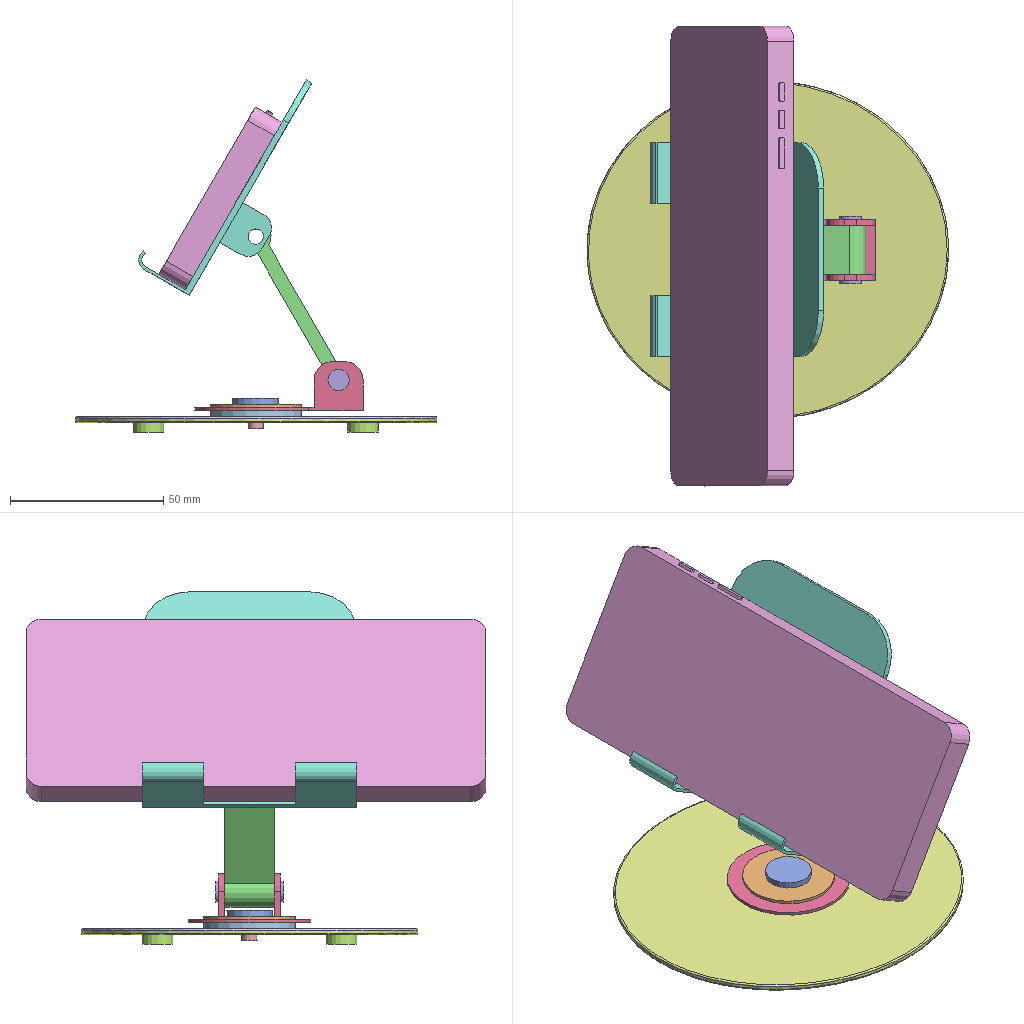Assembly | NX | 11 different items | 14 placed | box 118 x 150 x 115 mm
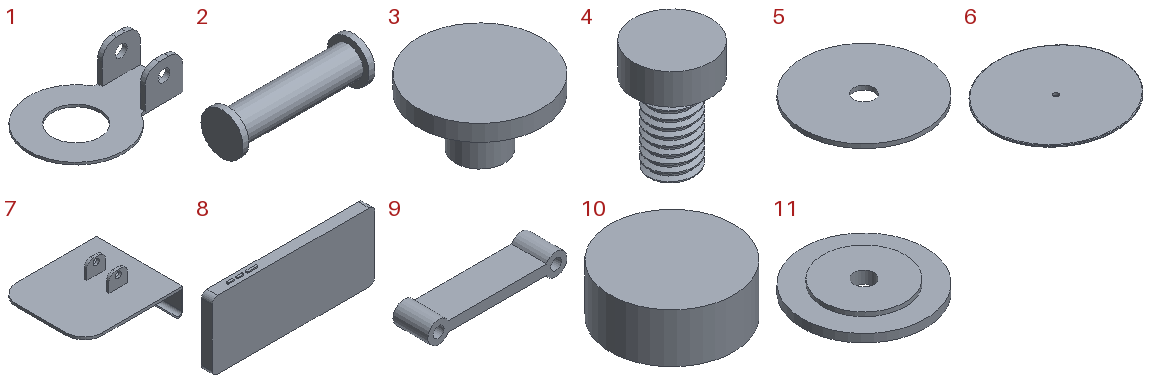Parts list (item | quantity | size | volume | features):
1 | x1 | 55 x 40 x 16 mm | 2079 mm3 | features DATUM_CSYS 5, EXTRUDE 4, SKETCH 4, BLEND 1
2 | x1 | 22 x 7 x 7 mm | 469.668 mm3 | features DATUM_CSYS 4, EXTRUDE 3, SKETCH 3
3 | x1 | 15 x 15 x 8 mm | 492.132 mm3 | features DATUM_CSYS 3, EXTRUDE 2, SKETCH 2, HOLE PACKAGE 1, SIMPLE HOLE 1, SYMBOLIC_THREAD 1
4 | x1 | 5 x 5 x 7 mm | 68.706 mm3 | features DATUM_CSYS 3, EXTRUDE 2, SKETCH 2, THREADS 1
5 | x1 | 30 x 30 x 1 mm | 687.223 mm3 | features DATUM_CSYS 2, EXTRUDE 1, SKETCH 1
6 | x1 | 118.002 x 110 x 2 mm | 20001 mm3 | features DATUM_CSYS 4, EXTRUDE 3, SKETCH 3, BLEND 1
7 | x1 | 80 x 70 x 33.5 mm | 12516 mm3 | features DATUM_CSYS 8, EXTRUDE 7, SKETCH 7, BLEND 2
8 | x1 | 150 x 10 x 64.04 mm | 94388 mm3 | features DATUM_CSYS 3, BLEND 2, EXTRUDE 2, SKETCH 2
9 | x1 | 64 x 16 x 10 mm | 5121 mm3 | features DATUM_CSYS 5, EXTRUDE 4, SKETCH 4
10 | x4 | 10 x 10 x 4 mm | 314.159 mm3 | features DATUM_CSYS 2, EXTRUDE 1, SKETCH 1
11 | x1 | 30 x 30 x 3 mm | 1669 mm3 | features DATUM_CSYS 4, EXTRUDE 3, SKETCH 3
Mates (type | each side: item.copy, entity, surface, feature):
Fix | 6.1 component
Concentric | 9.1 edge | 1.1 edge
Touch | 8.1 face plane Extrude(1) | 7.1 face plane Extrude(1)
Touch | 8.1 face plane Extrude(1) | 7.1 face plane Extrude(4)
Concentric | 3.1 edge | 5.1 edge
Concentric | 4.1 edge | 3.1 edge